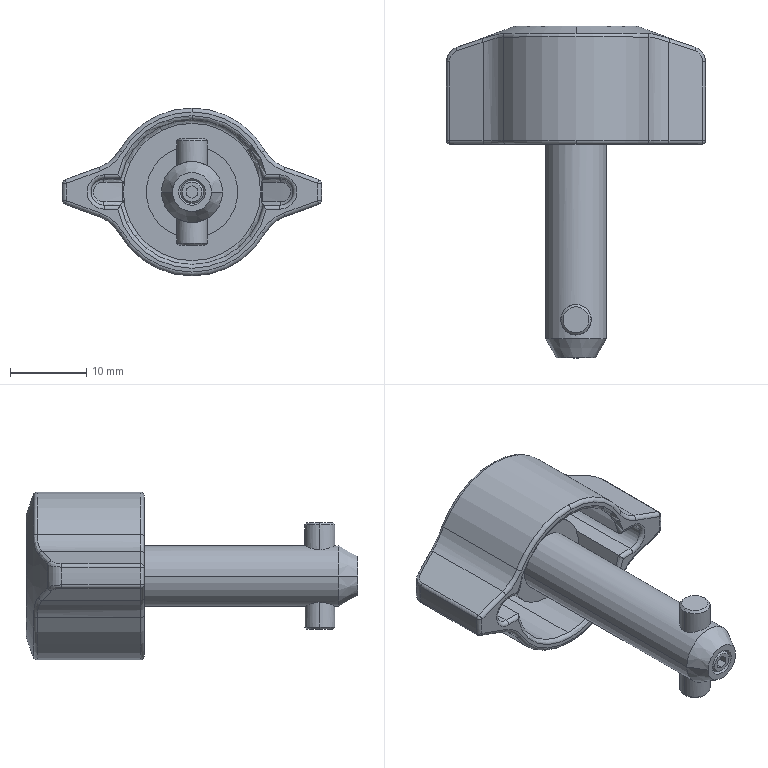Part | STEP file | QCTHA0834-14_02^qctha0834-14_FBDS-CS | 1 solid | 134 faces | box 34 x 43.5 x 22 mm | volume 5217 mm3 | cylinder 40 | plane 31 | torus 25 | spline 18 | cone 16 | sphere 4 | commonest cylinder face diameters 1 x12 4 x4 10 x4 19 x3 22 x3 3 x2